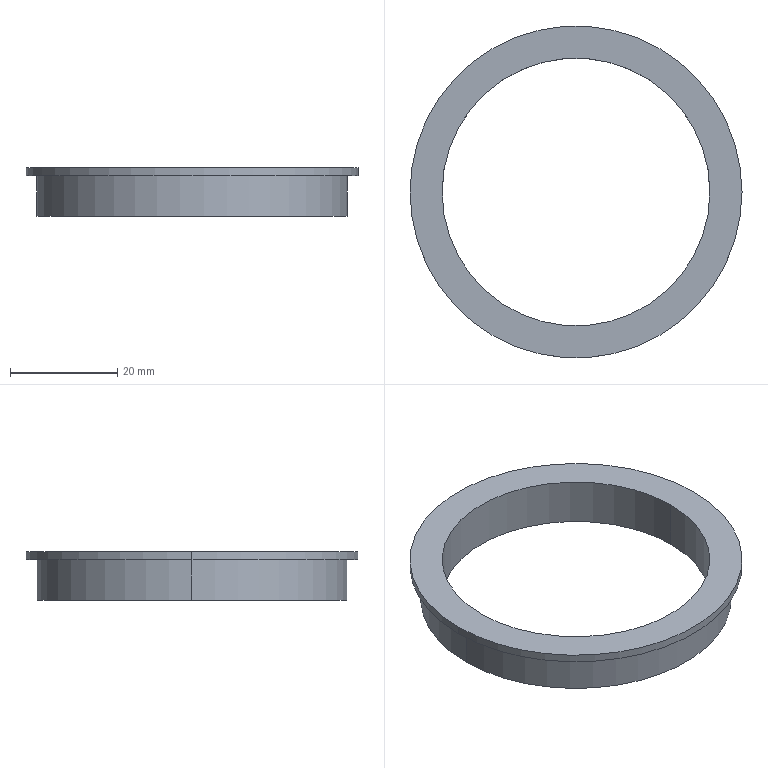Part | SolidWorks | features BaseBody 1 | 1 solid | 9 faces | box 62 x 62 x 9 mm | volume 6673 mm3 | cylinder 6 | plane 3 | commonest cylinder face diameters 50 x2 58 x2 62 x2
STEP:
#1=CARTESIAN_POINT('',(-25.,0.,3.));
#2=VERTEX_POINT('',#1);
#3=CARTESIAN_POINT('',(25.,0.,3.));
#4=VERTEX_POINT('',#3);
#5=CARTESIAN_POINT('',(0.,0.,3.));
#6=DIRECTION('',(0.,0.,1.));
#7=DIRECTION('',(1.,0.,0.));
#8=AXIS2_PLACEMENT_3D('',#5,#6,#7);
#9=CIRCLE('',#8,25.);
#10=EDGE_CURVE('',#2,#4,#9,.T.);
#11=ORIENTED_EDGE('',*,*,#10,.F.);
#12=CARTESIAN_POINT('',(-25.,0.,12.));
#13=VERTEX_POINT('',#12);
#14=CARTESIAN_POINT('',(-25.,0.,3.));
#15=DIRECTION('',(0.,0.,1.));
#16=VECTOR('',#15,1000.);
#17=LINE('',#14,#16);
#18=EDGE_CURVE('',#2,#13,#17,.T.);
#19=ORIENTED_EDGE('',*,*,#18,.T.);
#20=CARTESIAN_POINT('',(25.,0.,12.));
#21=VERTEX_POINT('',#20);
#22=CARTESIAN_POINT('',(0.,0.,12.));
#23=DIRECTION('',(0.,0.,-1.));
#24=DIRECTION('',(1.,0.,0.));
#25=AXIS2_PLACEMENT_3D('',#22,#23,#24);
#26=CIRCLE('',#25,25.);
#27=EDGE_CURVE('',#21,#13,#26,.T.);
#28=ORIENTED_EDGE('',*,*,#27,.F.);
#29=CARTESIAN_POINT('',(25.,0.,3.));
#30=DIRECTION('',(0.,0.,1.));
#31=VECTOR('',#30,1000.);
#32=LINE('',#29,#31);
#33=EDGE_CURVE('',#4,#21,#32,.T.);
#34=ORIENTED_EDGE('',*,*,#33,.F.);
#35=EDGE_LOOP('',(#11,#19,#28,#34));
#36=FACE_OUTER_BOUND('',#35,.T.);
#37=CARTESIAN_POINT('',(0.,0.,3.));
#38=DIRECTION('',(0.,0.,1.));
#39=DIRECTION('',(1.,0.,0.));
#40=AXIS2_PLACEMENT_3D('',#37,#38,#39);
#41=CYLINDRICAL_SURFACE('',#40,25.);
#42=ADVANCED_FACE('',(#36),#41,.F.);
#43=CARTESIAN_POINT('',(31.,0.,10.5));
#44=VERTEX_POINT('',#43);
#45=CARTESIAN_POINT('',(-31.,0.,10.5));
#46=VERTEX_POINT('',#45);
#47=CARTESIAN_POINT('',(0.,0.,10.5));
#48=DIRECTION('',(0.,0.,1.));
#49=DIRECTION('',(1.,0.,0.));
#50=AXIS2_PLACEMENT_3D('',#47,#48,#49);
#51=CIRCLE('',#50,31.);
#52=EDGE_CURVE('',#44,#46,#51,.T.);
#53=ORIENTED_EDGE('',*,*,#52,.T.);
#54=CARTESIAN_POINT('',(-31.,0.,12.));
#55=VERTEX_POINT('',#54);
#56=CARTESIAN_POINT('',(-31.,0.,10.5));
#57=DIRECTION('',(0.,0.,1.));
#58=VECTOR('',#57,1000.);
#59=LINE('',#56,#58);
#60=EDGE_CURVE('',#46,#55,#59,.T.);
#61=ORIENTED_EDGE('',*,*,#60,.T.);
#62=CARTESIAN_POINT('',(31.,0.,12.));
#63=VERTEX_POINT('',#62);
#64=CARTESIAN_POINT('',(0.,0.,12.));
#65=DIRECTION('',(0.,0.,1.));
#66=DIRECTION('',(1.,0.,0.));
#67=AXIS2_PLACEMENT_3D('',#64,#65,#66);
#68=CIRCLE('',#67,31.);
#69=EDGE_CURVE('',#63,#55,#68,.T.);
#70=ORIENTED_EDGE('',*,*,#69,.F.);
#71=CARTESIAN_POINT('',(31.,0.,10.5));
#72=DIRECTION('',(0.,0.,1.));
#73=VECTOR('',#72,1000.);
#74=LINE('',#71,#73);
#75=EDGE_CURVE('',#44,#63,#74,.T.);
#76=ORIENTED_EDGE('',*,*,#75,.F.);
#77=EDGE_LOOP('',(#53,#61,#70,#76));
#78=FACE_OUTER_BOUND('',#77,.T.);
#79=CARTESIAN_POINT('',(0.,0.,10.5));
#80=DIRECTION('',(0.,0.,1.));
#81=DIRECTION('',(1.,0.,0.));
#82=AXIS2_PLACEMENT_3D('',#79,#80,#81);
#83=CYLINDRICAL_SURFACE('',#82,31.);
#84=ADVANCED_FACE('',(#78),#83,.T.);
#85=CARTESIAN_POINT('',(29.,0.,3.));
#86=VERTEX_POINT('',#85);
#87=CARTESIAN_POINT('',(-29.,0.,3.));
#88=VERTEX_POINT('',#87);
#89=CARTESIAN_POINT('',(0.,0.,3.));
#90=DIRECTION('',(0.,0.,1.));
#91=DIRECTION('',(1.,0.,0.));
#92=AXIS2_PLACEMENT_3D('',#89,#90,#91);
#93=CIRCLE('',#92,29.);
#94=EDGE_CURVE('',#86,#88,#93,.T.);
#95=ORIENTED_EDGE('',*,*,#94,.T.);
#96=CARTESIAN_POINT('',(-29.,0.,10.5));
#97=VERTEX_POINT('',#96);
#98=CARTESIAN_POINT('',(-29.,0.,3.));
#99=DIRECTION('',(0.,0.,1.));
#100=VECTOR('',#99,1000.);
#101=LINE('',#98,#100);
#102=EDGE_CURVE('',#88,#97,#101,.T.);
#103=ORIENTED_EDGE('',*,*,#102,.T.);
#104=CARTESIAN_POINT('',(29.,0.,10.5));
#105=VERTEX_POINT('',#104);
#106=CARTESIAN_POINT('',(0.,0.,10.5));
#107=DIRECTION('',(0.,0.,-1.));
#108=DIRECTION('',(1.,0.,0.));
#109=AXIS2_PLACEMENT_3D('',#106,#107,#108);
#110=CIRCLE('',#109,29.);
#111=EDGE_CURVE('',#97,#105,#110,.T.);
#112=ORIENTED_EDGE('',*,*,#111,.T.);
#113=CARTESIAN_POINT('',(29.,0.,3.));
#114=DIRECTION('',(0.,0.,1.));
#115=VECTOR('',#114,1000.);
#116=LINE('',#113,#115);
#117=EDGE_CURVE('',#86,#105,#116,.T.);
#118=ORIENTED_EDGE('',*,*,#117,.F.);
#119=EDGE_LOOP('',(#95,#103,#112,#118));
#120=FACE_OUTER_BOUND('',#119,.T.);
#121=CARTESIAN_POINT('',(0.,0.,3.));
#122=DIRECTION('',(0.,0.,1.));
#123=DIRECTION('',(1.,0.,0.));
#124=AXIS2_PLACEMENT_3D('',#121,#122,#123);
#125=CYLINDRICAL_SURFACE('',#124,29.);
#126=ADVANCED_FACE('',(#120),#125,.T.);
#127=ORIENTED_EDGE('',*,*,#18,.F.);
#128=CARTESIAN_POINT('',(0.,0.,3.));
#129=DIRECTION('',(0.,0.,1.));
#130=DIRECTION('',(1.,0.,0.));
#131=AXIS2_PLACEMENT_3D('',#128,#129,#130);
#132=CIRCLE('',#131,25.);
#133=EDGE_CURVE('',#4,#2,#132,.T.);
#134=ORIENTED_EDGE('',*,*,#133,.F.);
#135=ORIENTED_EDGE('',*,*,#33,.T.);
#136=CARTESIAN_POINT('',(0.,0.,12.));
#137=DIRECTION('',(0.,0.,-1.));
#138=DIRECTION('',(1.,0.,0.));
#139=AXIS2_PLACEMENT_3D('',#136,#137,#138);
#140=CIRCLE('',#139,25.);
#141=EDGE_CURVE('',#13,#21,#140,.T.);
#142=ORIENTED_EDGE('',*,*,#141,.F.);
#143=EDGE_LOOP('',(#127,#134,#135,#142));
#144=FACE_OUTER_BOUND('',#143,.T.);
#145=CARTESIAN_POINT('',(0.,0.,3.));
#146=DIRECTION('',(0.,0.,1.));
#147=DIRECTION('',(1.,0.,0.));
#148=AXIS2_PLACEMENT_3D('',#145,#146,#147);
#149=CYLINDRICAL_SURFACE('',#148,25.);
#150=ADVANCED_FACE('',(#144),#149,.F.);
#151=ORIENTED_EDGE('',*,*,#27,.T.);
#152=ORIENTED_EDGE('',*,*,#141,.T.);
#153=EDGE_LOOP('',(#151,#152));
#154=FACE_BOUND('',#153,.T.);
#155=ORIENTED_EDGE('',*,*,#69,.T.);
#156=CARTESIAN_POINT('',(0.,0.,12.));
#157=DIRECTION('',(0.,0.,1.));
#158=DIRECTION('',(1.,0.,0.));
#159=AXIS2_PLACEMENT_3D('',#156,#157,#158);
#160=CIRCLE('',#159,31.);
#161=EDGE_CURVE('',#55,#63,#160,.T.);
#162=ORIENTED_EDGE('',*,*,#161,.T.);
#163=EDGE_LOOP('',(#155,#162));
#164=FACE_OUTER_BOUND('',#163,.T.);
#165=CARTESIAN_POINT('',(0.,0.,12.));
#166=DIRECTION('',(0.,0.,1.));
#167=DIRECTION('',(1.,0.,0.));
#168=AXIS2_PLACEMENT_3D('',#165,#166,#167);
#169=PLANE('',#168);
#170=ADVANCED_FACE('',(#154,#164),#169,.T.);
#171=ORIENTED_EDGE('',*,*,#133,.T.);
#172=ORIENTED_EDGE('',*,*,#10,.T.);
#173=EDGE_LOOP('',(#171,#172));
#174=FACE_BOUND('',#173,.T.);
#175=ORIENTED_EDGE('',*,*,#94,.F.);
#176=CARTESIAN_POINT('',(0.,0.,3.));
#177=DIRECTION('',(0.,0.,1.));
#178=DIRECTION('',(1.,0.,0.));
#179=AXIS2_PLACEMENT_3D('',#176,#177,#178);
#180=CIRCLE('',#179,29.);
#181=EDGE_CURVE('',#88,#86,#180,.T.);
#182=ORIENTED_EDGE('',*,*,#181,.F.);
#183=EDGE_LOOP('',(#175,#182));
#184=FACE_OUTER_BOUND('',#183,.T.);
#185=CARTESIAN_POINT('',(0.,0.,3.));
#186=DIRECTION('',(0.,0.,1.));
#187=DIRECTION('',(1.,0.,0.));
#188=AXIS2_PLACEMENT_3D('',#185,#186,#187);
#189=PLANE('',#188);
#190=ADVANCED_FACE('',(#174,#184),#189,.F.);
#191=ORIENTED_EDGE('',*,*,#60,.F.);
#192=CARTESIAN_POINT('',(0.,0.,10.5));
#193=DIRECTION('',(0.,0.,1.));
#194=DIRECTION('',(1.,0.,0.));
#195=AXIS2_PLACEMENT_3D('',#192,#193,#194);
#196=CIRCLE('',#195,31.);
#197=EDGE_CURVE('',#46,#44,#196,.T.);
#198=ORIENTED_EDGE('',*,*,#197,.T.);
#199=ORIENTED_EDGE('',*,*,#75,.T.);
#200=ORIENTED_EDGE('',*,*,#161,.F.);
#201=EDGE_LOOP('',(#191,#198,#199,#200));
#202=FACE_OUTER_BOUND('',#201,.T.);
#203=CARTESIAN_POINT('',(0.,0.,10.5));
#204=DIRECTION('',(0.,0.,1.));
#205=DIRECTION('',(1.,0.,0.));
#206=AXIS2_PLACEMENT_3D('',#203,#204,#205);
#207=CYLINDRICAL_SURFACE('',#206,31.);
#208=ADVANCED_FACE('',(#202),#207,.T.);
#209=ORIENTED_EDGE('',*,*,#102,.F.);
#210=ORIENTED_EDGE('',*,*,#181,.T.);
#211=ORIENTED_EDGE('',*,*,#117,.T.);
#212=CARTESIAN_POINT('',(0.,0.,10.5));
#213=DIRECTION('',(0.,0.,-1.));
#214=DIRECTION('',(1.,0.,0.));
#215=AXIS2_PLACEMENT_3D('',#212,#213,#214);
#216=CIRCLE('',#215,29.);
#217=EDGE_CURVE('',#105,#97,#216,.T.);
#218=ORIENTED_EDGE('',*,*,#217,.T.);
#219=EDGE_LOOP('',(#209,#210,#211,#218));
#220=FACE_OUTER_BOUND('',#219,.T.);
#221=CARTESIAN_POINT('',(0.,0.,3.));
#222=DIRECTION('',(0.,0.,1.));
#223=DIRECTION('',(1.,0.,0.));
#224=AXIS2_PLACEMENT_3D('',#221,#222,#223);
#225=CYLINDRICAL_SURFACE('',#224,29.);
#226=ADVANCED_FACE('',(#220),#225,.T.);
#227=ORIENTED_EDGE('',*,*,#217,.F.);
#228=ORIENTED_EDGE('',*,*,#111,.F.);
#229=EDGE_LOOP('',(#227,#228));
#230=FACE_BOUND('',#229,.T.);
#231=ORIENTED_EDGE('',*,*,#52,.F.);
#232=ORIENTED_EDGE('',*,*,#197,.F.);
#233=EDGE_LOOP('',(#231,#232));
#234=FACE_OUTER_BOUND('',#233,.T.);
#235=CARTESIAN_POINT('',(0.,0.,10.5));
#236=DIRECTION('',(0.,0.,1.));
#237=DIRECTION('',(1.,0.,0.));
#238=AXIS2_PLACEMENT_3D('',#235,#236,#237);
#239=PLANE('',#238);
#240=ADVANCED_FACE('',(#230,#234),#239,.F.);
#241=CLOSED_SHELL('',(#42,#84,#126,#150,#170,#190,#208,#226,#240));
#242=MANIFOLD_SOLID_BREP('',#241);
#243=CARTESIAN_POINT('',(0.,0.,0.));
#244=DIRECTION('',(0.,0.,1.));
#245=DIRECTION('',(1.,0.,0.));
#246=AXIS2_PLACEMENT_3D('',#243,#244,#245);
#247=(LENGTH_UNIT()NAMED_UNIT(*)SI_UNIT(.MILLI.,.METRE.));
#248=UNCERTAINTY_MEASURE_WITH_UNIT(LENGTH_MEASURE(0.00001),#247,'','');
#249=(NAMED_UNIT(*)PLANE_ANGLE_UNIT()SI_UNIT($,.RADIAN.));
#250=(NAMED_UNIT(*)SI_UNIT($,.STERADIAN.)SOLID_ANGLE_UNIT());
#251=(GEOMETRIC_REPRESENTATION_CONTEXT(3)GLOBAL_UNCERTAINTY_ASSIGNED_CONTEXT((#248))GLOBAL_UNIT_ASSIGNED_CONTEXT((#247,#249,#250))REPRESENTATION_CONTEXT('',''));
#252=ADVANCED_BREP_SHAPE_REPRESENTATION('',(#242,#246),#251);